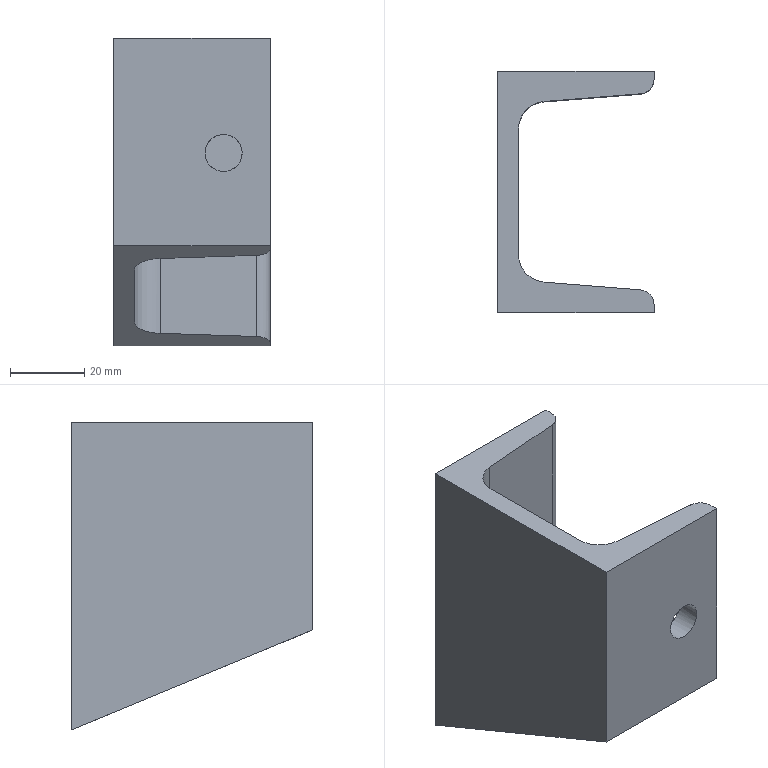Part | STEP file | DIN 1026-1 U 65 1785352380365 | 1 solid | 15 faces | box 42 x 65 x 82.843 mm | volume 62132 mm3 | plane 10 | cylinder 5 | commonest cylinder face diameters 8 x2 15 x2 10 x1
STEP:
#1=CARTESIAN_POINT('',(24.5,-32.5,51.924));
#2=VERTEX_POINT('',#1);
#3=CARTESIAN_POINT('',(29.5,-32.5,51.924));
#4=DIRECTION('',(0.,1.,0.));
#5=DIRECTION('',(1.,0.,0.));
#6=AXIS2_PLACEMENT_3D('',#3,#4,#5);
#7=CIRCLE('',#6,5.);
#8=EDGE_CURVE('',#2,#2,#7,.T.);
#9=ORIENTED_EDGE('',*,*,#8,.F.);
#10=CARTESIAN_POINT('',(24.5,-25.28,51.924));
#11=VERTEX_POINT('',#10);
#12=CARTESIAN_POINT('',(24.5,-32.5,51.924));
#13=DIRECTION('',(0.,1.,0.));
#14=VECTOR('',#13,5.);
#15=LINE('',#12,#14);
#16=EDGE_CURVE('',#2,#11,#15,.T.);
#17=ORIENTED_EDGE('',*,*,#16,.T.);
#18=CARTESIAN_POINT('',(29.5,-25.68,51.924));
#19=DIRECTION('',(-0.07975,-0.9968,0.));
#20=DIRECTION('',(0.9968,-0.07975,0.));
#21=AXIS2_PLACEMENT_3D('',#18,#19,#20);
#22=ELLIPSE('',#21,5.016,5.);
#23=EDGE_CURVE('',#11,#11,#22,.T.);
#24=ORIENTED_EDGE('',*,*,#23,.F.);
#25=ORIENTED_EDGE('',*,*,#16,.F.);
#26=EDGE_LOOP('',(#9,#17,#24,#25));
#27=FACE_OUTER_BOUND('',#26,.T.);
#28=CARTESIAN_POINT('',(29.5,-32.5,51.924));
#29=DIRECTION('',(0.,1.,0.));
#30=DIRECTION('',(1.,0.,0.));
#31=AXIS2_PLACEMENT_3D('',#28,#29,#30);
#32=CYLINDRICAL_SURFACE('',#31,5.);
#33=ADVANCED_FACE('',(#27),#32,.F.);
#34=CARTESIAN_POINT('',(12.402,-24.312,23.532));
#35=VERTEX_POINT('',#34);
#36=CARTESIAN_POINT('',(5.5,-16.836,20.436));
#37=VERTEX_POINT('',#36);
#38=CARTESIAN_POINT('',(13.,-16.836,20.436));
#39=DIRECTION('',(0.,-0.3827,-0.9239));
#40=DIRECTION('',(0.,-0.9239,0.3827));
#41=AXIS2_PLACEMENT_3D('',#38,#39,#40);
#42=ELLIPSE('',#41,8.118,7.5);
#43=EDGE_CURVE('',#35,#37,#42,.T.);
#44=ORIENTED_EDGE('',*,*,#43,.F.);
#45=CARTESIAN_POINT('',(38.319,-26.386,24.391));
#46=VERTEX_POINT('',#45);
#47=CARTESIAN_POINT('',(4.508,-23.681,23.271));
#48=DIRECTION('',(-0.9963,0.0797,-0.03301));
#49=VECTOR('',#48,10.);
#50=LINE('',#47,#49);
#51=EDGE_CURVE('',#46,#35,#50,.T.);
#52=ORIENTED_EDGE('',*,*,#51,.F.);
#53=CARTESIAN_POINT('',(42.,-30.373,26.043));
#54=VERTEX_POINT('',#53);
#55=CARTESIAN_POINT('',(38.,-30.373,26.043));
#56=DIRECTION('',(0.,0.3827,0.9239));
#57=DIRECTION('',(0.,-0.9239,0.3827));
#58=AXIS2_PLACEMENT_3D('',#55,#56,#57);
#59=ELLIPSE('',#58,4.33,4.);
#60=EDGE_CURVE('',#54,#46,#59,.T.);
#61=ORIENTED_EDGE('',*,*,#60,.F.);
#62=CARTESIAN_POINT('',(42.,-32.5,26.924));
#63=VERTEX_POINT('',#62);
#64=CARTESIAN_POINT('',(42.,-8.203,16.86));
#65=DIRECTION('',(0.,0.9239,-0.3827));
#66=VECTOR('',#65,10.);
#67=LINE('',#64,#66);
#68=EDGE_CURVE('',#63,#54,#67,.T.);
#69=ORIENTED_EDGE('',*,*,#68,.F.);
#70=CARTESIAN_POINT('',(0.,-32.5,26.924));
#71=VERTEX_POINT('',#70);
#72=CARTESIAN_POINT('',(21.,-32.5,26.924));
#73=DIRECTION('',(1.,0.,0.));
#74=VECTOR('',#73,10.);
#75=LINE('',#72,#74);
#76=EDGE_CURVE('',#71,#63,#75,.T.);
#77=ORIENTED_EDGE('',*,*,#76,.F.);
#78=CARTESIAN_POINT('',(0.,32.5,0.));
#79=VERTEX_POINT('',#78);
#80=CARTESIAN_POINT('',(0.,4.76,11.49));
#81=DIRECTION('',(0.,-0.9239,0.3827));
#82=VECTOR('',#81,10.);
#83=LINE('',#80,#82);
#84=EDGE_CURVE('',#79,#71,#83,.T.);
#85=ORIENTED_EDGE('',*,*,#84,.F.);
#86=CARTESIAN_POINT('',(42.,32.5,0.));
#87=VERTEX_POINT('',#86);
#88=CARTESIAN_POINT('',(10.5,32.5,0.));
#89=DIRECTION('',(1.,0.,0.));
#90=VECTOR('',#89,10.);
#91=LINE('',#88,#90);
#92=EDGE_CURVE('',#79,#87,#91,.T.);
#93=ORIENTED_EDGE('',*,*,#92,.T.);
#94=CARTESIAN_POINT('',(42.,30.373,0.8811));
#95=VERTEX_POINT('',#94);
#96=CARTESIAN_POINT('',(42.,18.63,5.745));
#97=DIRECTION('',(0.,0.9239,-0.3827));
#98=VECTOR('',#97,10.);
#99=LINE('',#96,#98);
#100=EDGE_CURVE('',#95,#87,#99,.T.);
#101=ORIENTED_EDGE('',*,*,#100,.F.);
#102=CARTESIAN_POINT('',(38.319,26.386,2.533));
#103=VERTEX_POINT('',#102);
#104=CARTESIAN_POINT('',(38.,30.373,0.8811));
#105=DIRECTION('',(0.,0.3827,0.9239));
#106=DIRECTION('',(0.,0.9239,-0.3827));
#107=AXIS2_PLACEMENT_3D('',#104,#105,#106);
#108=ELLIPSE('',#107,4.33,4.);
#109=EDGE_CURVE('',#103,#95,#108,.T.);
#110=ORIENTED_EDGE('',*,*,#109,.F.);
#111=CARTESIAN_POINT('',(12.402,24.312,3.392));
#112=VERTEX_POINT('',#111);
#113=CARTESIAN_POINT('',(18.338,24.787,3.195));
#114=DIRECTION('',(0.9963,0.0797,-0.03301));
#115=VECTOR('',#114,10.);
#116=LINE('',#113,#115);
#117=EDGE_CURVE('',#112,#103,#116,.T.);
#118=ORIENTED_EDGE('',*,*,#117,.F.);
#119=CARTESIAN_POINT('',(5.5,16.836,6.488));
#120=VERTEX_POINT('',#119);
#121=CARTESIAN_POINT('',(13.,16.836,6.488));
#122=DIRECTION('',(0.,-0.3827,-0.9239));
#123=DIRECTION('',(0.,0.9239,-0.3827));
#124=AXIS2_PLACEMENT_3D('',#121,#122,#123);
#125=ELLIPSE('',#124,8.118,7.5);
#126=EDGE_CURVE('',#120,#112,#125,.T.);
#127=ORIENTED_EDGE('',*,*,#126,.F.);
#128=CARTESIAN_POINT('',(5.5,4.76,11.49));
#129=DIRECTION('',(0.,0.9239,-0.3827));
#130=VECTOR('',#129,10.);
#131=LINE('',#128,#130);
#132=EDGE_CURVE('',#37,#120,#131,.T.);
#133=ORIENTED_EDGE('',*,*,#132,.F.);
#134=EDGE_LOOP('',(#44,#52,#61,#69,#77,#85,#93,#101,#110,#118,#127,#133));
#135=FACE_OUTER_BOUND('',#134,.T.);
#136=CARTESIAN_POINT('',(0.,4.76,11.49));
#137=DIRECTION('',(0.,0.3827,0.9239));
#138=DIRECTION('',(1.,0.,0.));
#139=AXIS2_PLACEMENT_3D('',#136,#137,#138);
#140=PLANE('',#139);
#141=ADVANCED_FACE('',(#135),#140,.F.);
#142=ORIENTED_EDGE('',*,*,#84,.T.);
#143=CARTESIAN_POINT('',(0.,-32.5,82.843));
#144=VERTEX_POINT('',#143);
#145=CARTESIAN_POINT('',(0.,-32.5,0.));
#146=DIRECTION('',(0.,0.,1.));
#147=VECTOR('',#146,10.);
#148=LINE('',#145,#147);
#149=EDGE_CURVE('',#71,#144,#148,.T.);
#150=ORIENTED_EDGE('',*,*,#149,.T.);
#151=CARTESIAN_POINT('',(0.,32.5,82.843));
#152=VERTEX_POINT('',#151);
#153=CARTESIAN_POINT('',(0.,0.,82.843));
#154=DIRECTION('',(0.,1.,0.));
#155=VECTOR('',#154,10.);
#156=LINE('',#153,#155);
#157=EDGE_CURVE('',#144,#152,#156,.T.);
#158=ORIENTED_EDGE('',*,*,#157,.T.);
#159=CARTESIAN_POINT('',(0.,32.5,0.));
#160=DIRECTION('',(0.,0.,1.));
#161=VECTOR('',#160,10.);
#162=LINE('',#159,#161);
#163=EDGE_CURVE('',#79,#152,#162,.T.);
#164=ORIENTED_EDGE('',*,*,#163,.F.);
#165=EDGE_LOOP('',(#142,#150,#158,#164));
#166=FACE_OUTER_BOUND('',#165,.T.);
#167=CARTESIAN_POINT('',(0.,0.,0.));
#168=DIRECTION('',(-1.,0.,0.));
#169=DIRECTION('',(0.,0.,1.));
#170=AXIS2_PLACEMENT_3D('',#167,#168,#169);
#171=PLANE('',#170);
#172=ADVANCED_FACE('',(#166),#171,.T.);
#173=ORIENTED_EDGE('',*,*,#76,.T.);
#174=CARTESIAN_POINT('',(42.,-32.5,82.843));
#175=VERTEX_POINT('',#174);
#176=CARTESIAN_POINT('',(42.,-32.5,0.));
#177=DIRECTION('',(0.,0.,1.));
#178=VECTOR('',#177,10.);
#179=LINE('',#176,#178);
#180=EDGE_CURVE('',#63,#175,#179,.T.);
#181=ORIENTED_EDGE('',*,*,#180,.T.);
#182=CARTESIAN_POINT('',(31.5,-32.5,82.843));
#183=DIRECTION('',(-1.,0.,0.));
#184=VECTOR('',#183,10.);
#185=LINE('',#182,#184);
#186=EDGE_CURVE('',#175,#144,#185,.T.);
#187=ORIENTED_EDGE('',*,*,#186,.T.);
#188=ORIENTED_EDGE('',*,*,#149,.F.);
#189=EDGE_LOOP('',(#173,#181,#187,#188));
#190=FACE_OUTER_BOUND('',#189,.T.);
#191=ORIENTED_EDGE('',*,*,#8,.T.);
#192=EDGE_LOOP('',(#191));
#193=FACE_BOUND('',#192,.T.);
#194=CARTESIAN_POINT('',(42.,-32.5,0.));
#195=DIRECTION('',(0.,-1.,0.));
#196=DIRECTION('',(0.,0.,-1.));
#197=AXIS2_PLACEMENT_3D('',#194,#195,#196);
#198=PLANE('',#197);
#199=ADVANCED_FACE('',(#190,#193),#198,.T.);
#200=ORIENTED_EDGE('',*,*,#68,.T.);
#201=CARTESIAN_POINT('',(42.,-30.373,82.843));
#202=VERTEX_POINT('',#201);
#203=CARTESIAN_POINT('',(42.,-30.373,0.));
#204=DIRECTION('',(0.,0.,1.));
#205=VECTOR('',#204,10.);
#206=LINE('',#203,#205);
#207=EDGE_CURVE('',#54,#202,#206,.T.);
#208=ORIENTED_EDGE('',*,*,#207,.T.);
#209=CARTESIAN_POINT('',(42.,-15.186,82.843));
#210=DIRECTION('',(0.,-1.,0.));
#211=VECTOR('',#210,10.);
#212=LINE('',#209,#211);
#213=EDGE_CURVE('',#202,#175,#212,.T.);
#214=ORIENTED_EDGE('',*,*,#213,.T.);
#215=ORIENTED_EDGE('',*,*,#180,.F.);
#216=EDGE_LOOP('',(#200,#208,#214,#215));
#217=FACE_OUTER_BOUND('',#216,.T.);
#218=CARTESIAN_POINT('',(42.,-30.373,0.));
#219=DIRECTION('',(1.,0.,0.));
#220=DIRECTION('',(0.,0.,-1.));
#221=AXIS2_PLACEMENT_3D('',#218,#219,#220);
#222=PLANE('',#221);
#223=ADVANCED_FACE('',(#217),#222,.T.);
#224=ORIENTED_EDGE('',*,*,#60,.T.);
#225=CARTESIAN_POINT('',(38.319,-26.386,82.843));
#226=VERTEX_POINT('',#225);
#227=CARTESIAN_POINT('',(38.319,-26.386,0.));
#228=DIRECTION('',(0.,0.,1.));
#229=VECTOR('',#228,10.);
#230=LINE('',#227,#229);
#231=EDGE_CURVE('',#46,#226,#230,.T.);
#232=ORIENTED_EDGE('',*,*,#231,.T.);
#233=CARTESIAN_POINT('',(38.,-30.373,82.843));
#234=DIRECTION('',(0.,0.,-1.));
#235=DIRECTION('',(-1.,0.,0.));
#236=AXIS2_PLACEMENT_3D('',#233,#234,#235);
#237=CIRCLE('',#236,4.);
#238=EDGE_CURVE('',#226,#202,#237,.T.);
#239=ORIENTED_EDGE('',*,*,#238,.T.);
#240=ORIENTED_EDGE('',*,*,#207,.F.);
#241=EDGE_LOOP('',(#224,#232,#239,#240));
#242=FACE_OUTER_BOUND('',#241,.T.);
#243=CARTESIAN_POINT('',(38.,-30.373,0.));
#244=DIRECTION('',(0.,0.,1.));
#245=DIRECTION('',(-1.,0.,0.));
#246=AXIS2_PLACEMENT_3D('',#243,#244,#245);
#247=CYLINDRICAL_SURFACE('',#246,4.);
#248=ADVANCED_FACE('',(#242),#247,.T.);
#249=ORIENTED_EDGE('',*,*,#51,.T.);
#250=CARTESIAN_POINT('',(12.402,-24.312,82.843));
#251=VERTEX_POINT('',#250);
#252=CARTESIAN_POINT('',(12.402,-24.312,0.));
#253=DIRECTION('',(0.,0.,1.));
#254=VECTOR('',#253,10.);
#255=LINE('',#252,#254);
#256=EDGE_CURVE('',#35,#251,#255,.T.);
#257=ORIENTED_EDGE('',*,*,#256,.T.);
#258=CARTESIAN_POINT('',(15.707,-24.577,82.843));
#259=DIRECTION('',(0.9968,-0.07975,0.));
#260=VECTOR('',#259,10.);
#261=LINE('',#258,#260);
#262=EDGE_CURVE('',#251,#226,#261,.T.);
#263=ORIENTED_EDGE('',*,*,#262,.T.);
#264=ORIENTED_EDGE('',*,*,#231,.F.);
#265=EDGE_LOOP('',(#249,#257,#263,#264));
#266=FACE_OUTER_BOUND('',#265,.T.);
#267=ORIENTED_EDGE('',*,*,#23,.T.);
#268=EDGE_LOOP('',(#267));
#269=FACE_BOUND('',#268,.T.);
#270=CARTESIAN_POINT('',(12.402,-24.312,0.));
#271=DIRECTION('',(0.07975,0.9968,0.));
#272=DIRECTION('',(0.,0.,1.));
#273=AXIS2_PLACEMENT_3D('',#270,#271,#272);
#274=PLANE('',#273);
#275=ADVANCED_FACE('',(#266,#269),#274,.T.);
#276=ORIENTED_EDGE('',*,*,#43,.T.);
#277=CARTESIAN_POINT('',(5.5,-16.836,82.843));
#278=VERTEX_POINT('',#277);
#279=CARTESIAN_POINT('',(5.5,-16.836,0.));
#280=DIRECTION('',(0.,0.,1.));
#281=VECTOR('',#280,10.);
#282=LINE('',#279,#281);
#283=EDGE_CURVE('',#37,#278,#282,.T.);
#284=ORIENTED_EDGE('',*,*,#283,.T.);
#285=CARTESIAN_POINT('',(13.,-16.836,82.843));
#286=DIRECTION('',(0.,0.,1.));
#287=DIRECTION('',(-1.,0.,0.));
#288=AXIS2_PLACEMENT_3D('',#285,#286,#287);
#289=CIRCLE('',#288,7.5);
#290=EDGE_CURVE('',#278,#251,#289,.T.);
#291=ORIENTED_EDGE('',*,*,#290,.T.);
#292=ORIENTED_EDGE('',*,*,#256,.F.);
#293=EDGE_LOOP('',(#276,#284,#291,#292));
#294=FACE_OUTER_BOUND('',#293,.T.);
#295=CARTESIAN_POINT('',(13.,-16.836,0.));
#296=DIRECTION('',(0.,0.,1.));
#297=DIRECTION('',(-1.,0.,0.));
#298=AXIS2_PLACEMENT_3D('',#295,#296,#297);
#299=CYLINDRICAL_SURFACE('',#298,7.5);
#300=ADVANCED_FACE('',(#294),#299,.F.);
#301=CARTESIAN_POINT('',(42.,32.5,82.843));
#302=VERTEX_POINT('',#301);
#303=CARTESIAN_POINT('',(10.5,32.5,82.843));
#304=DIRECTION('',(1.,0.,0.));
#305=VECTOR('',#304,10.);
#306=LINE('',#303,#305);
#307=EDGE_CURVE('',#152,#302,#306,.T.);
#308=ORIENTED_EDGE('',*,*,#307,.T.);
#309=CARTESIAN_POINT('',(42.,32.5,0.));
#310=DIRECTION('',(0.,0.,1.));
#311=VECTOR('',#310,10.);
#312=LINE('',#309,#311);
#313=EDGE_CURVE('',#87,#302,#312,.T.);
#314=ORIENTED_EDGE('',*,*,#313,.F.);
#315=ORIENTED_EDGE('',*,*,#92,.F.);
#316=ORIENTED_EDGE('',*,*,#163,.T.);
#317=EDGE_LOOP('',(#308,#314,#315,#316));
#318=FACE_OUTER_BOUND('',#317,.T.);
#319=CARTESIAN_POINT('',(0.,32.5,0.));
#320=DIRECTION('',(0.,1.,0.));
#321=DIRECTION('',(0.,0.,1.));
#322=AXIS2_PLACEMENT_3D('',#319,#320,#321);
#323=PLANE('',#322);
#324=ADVANCED_FACE('',(#318),#323,.T.);
#325=ORIENTED_EDGE('',*,*,#100,.T.);
#326=ORIENTED_EDGE('',*,*,#313,.T.);
#327=CARTESIAN_POINT('',(42.,30.373,82.843));
#328=VERTEX_POINT('',#327);
#329=CARTESIAN_POINT('',(42.,16.25,82.843));
#330=DIRECTION('',(0.,-1.,0.));
#331=VECTOR('',#330,10.);
#332=LINE('',#329,#331);
#333=EDGE_CURVE('',#302,#328,#332,.T.);
#334=ORIENTED_EDGE('',*,*,#333,.T.);
#335=CARTESIAN_POINT('',(42.,30.373,0.));
#336=DIRECTION('',(0.,0.,1.));
#337=VECTOR('',#336,10.);
#338=LINE('',#335,#337);
#339=EDGE_CURVE('',#95,#328,#338,.T.);
#340=ORIENTED_EDGE('',*,*,#339,.F.);
#341=EDGE_LOOP('',(#325,#326,#334,#340));
#342=FACE_OUTER_BOUND('',#341,.T.);
#343=CARTESIAN_POINT('',(42.,32.5,0.));
#344=DIRECTION('',(1.,0.,0.));
#345=DIRECTION('',(0.,0.,-1.));
#346=AXIS2_PLACEMENT_3D('',#343,#344,#345);
#347=PLANE('',#346);
#348=ADVANCED_FACE('',(#342),#347,.T.);
#349=ORIENTED_EDGE('',*,*,#109,.T.);
#350=ORIENTED_EDGE('',*,*,#339,.T.);
#351=CARTESIAN_POINT('',(38.319,26.386,82.843));
#352=VERTEX_POINT('',#351);
#353=CARTESIAN_POINT('',(38.,30.373,82.843));
#354=DIRECTION('',(0.,0.,-1.));
#355=DIRECTION('',(-0.07975,0.9968,0.));
#356=AXIS2_PLACEMENT_3D('',#353,#354,#355);
#357=CIRCLE('',#356,4.);
#358=EDGE_CURVE('',#328,#352,#357,.T.);
#359=ORIENTED_EDGE('',*,*,#358,.T.);
#360=CARTESIAN_POINT('',(38.319,26.386,0.));
#361=DIRECTION('',(0.,0.,1.));
#362=VECTOR('',#361,10.);
#363=LINE('',#360,#362);
#364=EDGE_CURVE('',#103,#352,#363,.T.);
#365=ORIENTED_EDGE('',*,*,#364,.F.);
#366=EDGE_LOOP('',(#349,#350,#359,#365));
#367=FACE_OUTER_BOUND('',#366,.T.);
#368=CARTESIAN_POINT('',(38.,30.373,0.));
#369=DIRECTION('',(0.,0.,1.));
#370=DIRECTION('',(-0.07975,0.9968,0.));
#371=AXIS2_PLACEMENT_3D('',#368,#369,#370);
#372=CYLINDRICAL_SURFACE('',#371,4.);
#373=ADVANCED_FACE('',(#367),#372,.T.);
#374=ORIENTED_EDGE('',*,*,#117,.T.);
#375=ORIENTED_EDGE('',*,*,#364,.T.);
#376=CARTESIAN_POINT('',(12.402,24.312,82.843));
#377=VERTEX_POINT('',#376);
#378=CARTESIAN_POINT('',(28.666,25.613,82.843));
#379=DIRECTION('',(-0.9968,-0.07975,0.));
#380=VECTOR('',#379,10.);
#381=LINE('',#378,#380);
#382=EDGE_CURVE('',#352,#377,#381,.T.);
#383=ORIENTED_EDGE('',*,*,#382,.T.);
#384=CARTESIAN_POINT('',(12.402,24.312,0.));
#385=DIRECTION('',(0.,0.,1.));
#386=VECTOR('',#385,10.);
#387=LINE('',#384,#386);
#388=EDGE_CURVE('',#112,#377,#387,.T.);
#389=ORIENTED_EDGE('',*,*,#388,.F.);
#390=EDGE_LOOP('',(#374,#375,#383,#389));
#391=FACE_OUTER_BOUND('',#390,.T.);
#392=CARTESIAN_POINT('',(38.319,26.386,0.));
#393=DIRECTION('',(0.07975,-0.9968,0.));
#394=DIRECTION('',(0.,0.,-1.));
#395=AXIS2_PLACEMENT_3D('',#392,#393,#394);
#396=PLANE('',#395);
#397=ADVANCED_FACE('',(#391),#396,.T.);
#398=ORIENTED_EDGE('',*,*,#126,.T.);
#399=ORIENTED_EDGE('',*,*,#388,.T.);
#400=CARTESIAN_POINT('',(5.5,16.836,82.843));
#401=VERTEX_POINT('',#400);
#402=CARTESIAN_POINT('',(13.,16.836,82.843));
#403=DIRECTION('',(0.,0.,1.));
#404=DIRECTION('',(-0.07975,0.9968,0.));
#405=AXIS2_PLACEMENT_3D('',#402,#403,#404);
#406=CIRCLE('',#405,7.5);
#407=EDGE_CURVE('',#377,#401,#406,.T.);
#408=ORIENTED_EDGE('',*,*,#407,.T.);
#409=CARTESIAN_POINT('',(5.5,16.836,0.));
#410=DIRECTION('',(0.,0.,1.));
#411=VECTOR('',#410,10.);
#412=LINE('',#409,#411);
#413=EDGE_CURVE('',#120,#401,#412,.T.);
#414=ORIENTED_EDGE('',*,*,#413,.F.);
#415=EDGE_LOOP('',(#398,#399,#408,#414));
#416=FACE_OUTER_BOUND('',#415,.T.);
#417=CARTESIAN_POINT('',(13.,16.836,0.));
#418=DIRECTION('',(0.,0.,1.));
#419=DIRECTION('',(-0.07975,0.9968,0.));
#420=AXIS2_PLACEMENT_3D('',#417,#418,#419);
#421=CYLINDRICAL_SURFACE('',#420,7.5);
#422=ADVANCED_FACE('',(#416),#421,.F.);
#423=ORIENTED_EDGE('',*,*,#132,.T.);
#424=ORIENTED_EDGE('',*,*,#413,.T.);
#425=CARTESIAN_POINT('',(5.5,0.,82.843));
#426=DIRECTION('',(0.,-1.,0.));
#427=VECTOR('',#426,10.);
#428=LINE('',#425,#427);
#429=EDGE_CURVE('',#401,#278,#428,.T.);
#430=ORIENTED_EDGE('',*,*,#429,.T.);
#431=ORIENTED_EDGE('',*,*,#283,.F.);
#432=EDGE_LOOP('',(#423,#424,#430,#431));
#433=FACE_OUTER_BOUND('',#432,.T.);
#434=CARTESIAN_POINT('',(5.5,0.,0.));
#435=DIRECTION('',(1.,0.,0.));
#436=DIRECTION('',(0.,0.,-1.));
#437=AXIS2_PLACEMENT_3D('',#434,#435,#436);
#438=PLANE('',#437);
#439=ADVANCED_FACE('',(#433),#438,.T.);
#440=ORIENTED_EDGE('',*,*,#307,.F.);
#441=ORIENTED_EDGE('',*,*,#157,.F.);
#442=ORIENTED_EDGE('',*,*,#186,.F.);
#443=ORIENTED_EDGE('',*,*,#213,.F.);
#444=ORIENTED_EDGE('',*,*,#238,.F.);
#445=ORIENTED_EDGE('',*,*,#262,.F.);
#446=ORIENTED_EDGE('',*,*,#290,.F.);
#447=ORIENTED_EDGE('',*,*,#429,.F.);
#448=ORIENTED_EDGE('',*,*,#407,.F.);
#449=ORIENTED_EDGE('',*,*,#382,.F.);
#450=ORIENTED_EDGE('',*,*,#358,.F.);
#451=ORIENTED_EDGE('',*,*,#333,.F.);
#452=EDGE_LOOP('',(#440,#441,#442,#443,#444,#445,#446,#447,#448,#449,#450,#451));
#453=FACE_OUTER_BOUND('',#452,.T.);
#454=CARTESIAN_POINT('',(21.,0.,82.843));
#455=DIRECTION('',(0.,0.,1.));
#456=DIRECTION('',(1.,0.,0.));
#457=AXIS2_PLACEMENT_3D('',#454,#455,#456);
#458=PLANE('',#457);
#459=ADVANCED_FACE('',(#453),#458,.T.);
#460=CLOSED_SHELL('',(#33,#141,#172,#199,#223,#248,#275,#300,#324,#348,#373,#397,#422,#439,#459));
#461=MANIFOLD_SOLID_BREP('',#460);
#462=(LENGTH_UNIT()NAMED_UNIT(*)SI_UNIT(.MILLI.,.METRE.));
#463=UNCERTAINTY_MEASURE_WITH_UNIT(LENGTH_MEASURE(0.01),#462,'','');
#464=(NAMED_UNIT(*)PLANE_ANGLE_UNIT()SI_UNIT($,.RADIAN.));
#465=(NAMED_UNIT(*)SI_UNIT($,.STERADIAN.)SOLID_ANGLE_UNIT());
#466=(GEOMETRIC_REPRESENTATION_CONTEXT(3)GLOBAL_UNCERTAINTY_ASSIGNED_CONTEXT((#463))GLOBAL_UNIT_ASSIGNED_CONTEXT((#462,#464,#465))REPRESENTATION_CONTEXT('',''));
#467=ADVANCED_BREP_SHAPE_REPRESENTATION('',(#461),#466);